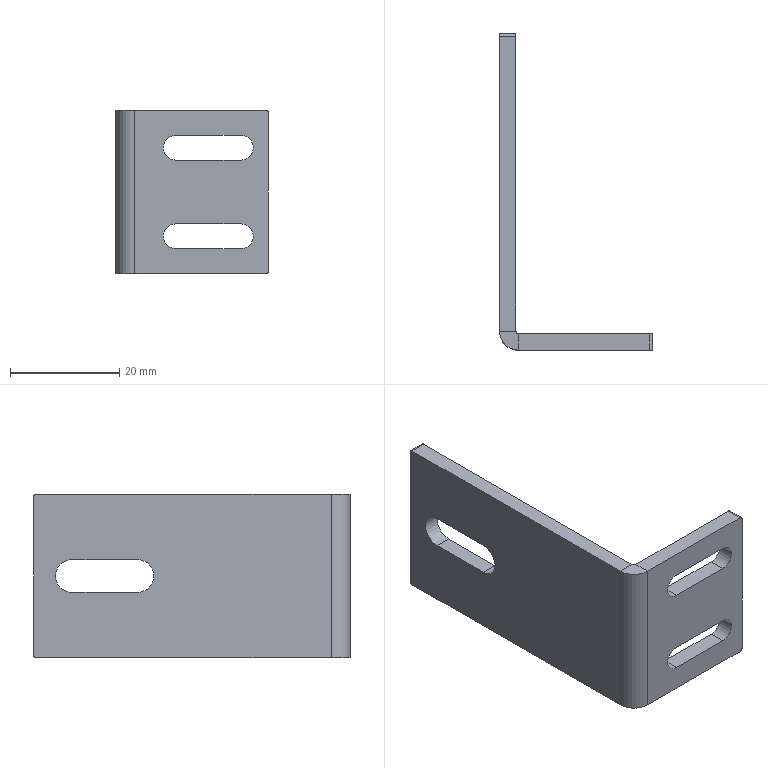Part | SolidWorks | features ICE 2, Fillet 1, FlatPattern 1, SMBaseFlange 1, SheetMetal 1 | 1 solid | 30 faces | box 28 x 58 x 30 mm | volume 6672 mm3 | plane 18 | cylinder 12 | commonest cylinder face diameters 1 x5 4.5 x4 6 x2 7 x1
STEP:
#1=CARTESIAN_POINT('',(0.5,0.,30.));
#2=VERTEX_POINT('',#1);
#3=CARTESIAN_POINT('',(0.5,-3.,30.));
#4=VERTEX_POINT('',#3);
#5=CARTESIAN_POINT('',(0.5,0.,30.));
#6=DIRECTION('',(0.,-1.,0.));
#7=VECTOR('',#6,1000.);
#8=LINE('',#5,#7);
#9=EDGE_CURVE('',#2,#4,#8,.T.);
#10=ORIENTED_EDGE('',*,*,#9,.F.);
#11=CARTESIAN_POINT('',(0.,0.5,30.));
#12=VERTEX_POINT('',#11);
#13=CARTESIAN_POINT('',(0.5,0.5,30.));
#14=DIRECTION('',(0.,0.,1.));
#15=DIRECTION('',(-1.,0.,0.));
#16=AXIS2_PLACEMENT_3D('',#13,#14,#15);
#17=CIRCLE('',#16,0.5);
#18=EDGE_CURVE('',#12,#2,#17,.T.);
#19=ORIENTED_EDGE('',*,*,#18,.F.);
#20=CARTESIAN_POINT('',(-3.,0.5,30.));
#21=VERTEX_POINT('',#20);
#22=CARTESIAN_POINT('',(-3.,0.5,30.));
#23=DIRECTION('',(1.,0.,0.));
#24=VECTOR('',#23,1000.);
#25=LINE('',#22,#24);
#26=EDGE_CURVE('',#21,#12,#25,.T.);
#27=ORIENTED_EDGE('',*,*,#26,.F.);
#28=CARTESIAN_POINT('',(0.5,0.5,30.));
#29=DIRECTION('',(0.,0.,1.));
#30=DIRECTION('',(1.,0.,0.));
#31=AXIS2_PLACEMENT_3D('',#28,#29,#30);
#32=CIRCLE('',#31,3.5);
#33=EDGE_CURVE('',#21,#4,#32,.T.);
#34=ORIENTED_EDGE('',*,*,#33,.T.);
#35=EDGE_LOOP('',(#10,#19,#27,#34));
#36=FACE_OUTER_BOUND('',#35,.T.);
#37=CARTESIAN_POINT('',(0.5,0.,30.));
#38=DIRECTION('',(0.,0.,1.));
#39=DIRECTION('',(1.,0.,0.));
#40=AXIS2_PLACEMENT_3D('',#37,#38,#39);
#41=PLANE('',#40);
#42=ADVANCED_FACE('',(#36),#41,.T.);
#43=CARTESIAN_POINT('',(24.5,-3.,30.));
#44=VERTEX_POINT('',#43);
#45=CARTESIAN_POINT('',(0.,-3.,30.));
#46=DIRECTION('',(1.,0.,0.));
#47=VECTOR('',#46,1000.);
#48=LINE('',#45,#47);
#49=EDGE_CURVE('',#4,#44,#48,.T.);
#50=ORIENTED_EDGE('',*,*,#49,.T.);
#51=CARTESIAN_POINT('',(24.5,0.,30.));
#52=VERTEX_POINT('',#51);
#53=CARTESIAN_POINT('',(24.5,0.5,30.));
#54=DIRECTION('',(0.,1.,0.));
#55=VECTOR('',#54,1000.);
#56=LINE('',#53,#55);
#57=EDGE_CURVE('',#44,#52,#56,.T.);
#58=ORIENTED_EDGE('',*,*,#57,.T.);
#59=CARTESIAN_POINT('',(0.,0.,30.));
#60=DIRECTION('',(1.,0.,0.));
#61=VECTOR('',#60,1000.);
#62=LINE('',#59,#61);
#63=EDGE_CURVE('',#2,#52,#62,.T.);
#64=ORIENTED_EDGE('',*,*,#63,.F.);
#65=ORIENTED_EDGE('',*,*,#9,.T.);
#66=EDGE_LOOP('',(#50,#58,#64,#65));
#67=FACE_OUTER_BOUND('',#66,.T.);
#68=CARTESIAN_POINT('',(-3.,0.5,30.));
#69=DIRECTION('',(0.,0.,1.));
#70=DIRECTION('',(1.,0.,0.));
#71=AXIS2_PLACEMENT_3D('',#68,#69,#70);
#72=PLANE('',#71);
#73=ADVANCED_FACE('',(#67),#72,.T.);
#74=CARTESIAN_POINT('',(0.,0.5,0.));
#75=VERTEX_POINT('',#74);
#76=CARTESIAN_POINT('',(-3.,0.5,0.));
#77=VERTEX_POINT('',#76);
#78=CARTESIAN_POINT('',(0.,0.5,0.));
#79=DIRECTION('',(-1.,0.,0.));
#80=VECTOR('',#79,1000.);
#81=LINE('',#78,#80);
#82=EDGE_CURVE('',#75,#77,#81,.T.);
#83=ORIENTED_EDGE('',*,*,#82,.F.);
#84=CARTESIAN_POINT('',(0.5,0.,0.));
#85=VERTEX_POINT('',#84);
#86=CARTESIAN_POINT('',(0.5,0.5,0.));
#87=DIRECTION('',(0.,0.,1.));
#88=DIRECTION('',(-1.,0.,0.));
#89=AXIS2_PLACEMENT_3D('',#86,#87,#88);
#90=CIRCLE('',#89,0.5);
#91=EDGE_CURVE('',#75,#85,#90,.T.);
#92=ORIENTED_EDGE('',*,*,#91,.T.);
#93=CARTESIAN_POINT('',(0.5,-3.,0.));
#94=VERTEX_POINT('',#93);
#95=CARTESIAN_POINT('',(0.5,-3.,0.));
#96=DIRECTION('',(0.,1.,0.));
#97=VECTOR('',#96,1000.);
#98=LINE('',#95,#97);
#99=EDGE_CURVE('',#94,#85,#98,.T.);
#100=ORIENTED_EDGE('',*,*,#99,.F.);
#101=CARTESIAN_POINT('',(0.5,0.5,0.));
#102=DIRECTION('',(0.,0.,1.));
#103=DIRECTION('',(1.,0.,0.));
#104=AXIS2_PLACEMENT_3D('',#101,#102,#103);
#105=CIRCLE('',#104,3.5);
#106=EDGE_CURVE('',#77,#94,#105,.T.);
#107=ORIENTED_EDGE('',*,*,#106,.F.);
#108=EDGE_LOOP('',(#83,#92,#100,#107));
#109=FACE_OUTER_BOUND('',#108,.T.);
#110=CARTESIAN_POINT('',(0.,0.5,0.));
#111=DIRECTION('',(0.,0.,-1.));
#112=DIRECTION('',(-1.,0.,0.));
#113=AXIS2_PLACEMENT_3D('',#110,#111,#112);
#114=PLANE('',#113);
#115=ADVANCED_FACE('',(#109),#114,.T.);
#116=CARTESIAN_POINT('',(-3.,54.5,0.));
#117=VERTEX_POINT('',#116);
#118=CARTESIAN_POINT('',(-3.,0.,0.));
#119=DIRECTION('',(0.,-1.,0.));
#120=VECTOR('',#119,1000.);
#121=LINE('',#118,#120);
#122=EDGE_CURVE('',#117,#77,#121,.T.);
#123=ORIENTED_EDGE('',*,*,#122,.F.);
#124=CARTESIAN_POINT('',(0.,54.5,0.));
#125=VERTEX_POINT('',#124);
#126=CARTESIAN_POINT('',(0.5,54.5,0.));
#127=DIRECTION('',(1.,0.,0.));
#128=VECTOR('',#127,1000.);
#129=LINE('',#126,#128);
#130=EDGE_CURVE('',#117,#125,#129,.T.);
#131=ORIENTED_EDGE('',*,*,#130,.T.);
#132=CARTESIAN_POINT('',(0.,0.,0.));
#133=DIRECTION('',(0.,-1.,0.));
#134=VECTOR('',#133,1000.);
#135=LINE('',#132,#134);
#136=EDGE_CURVE('',#125,#75,#135,.T.);
#137=ORIENTED_EDGE('',*,*,#136,.T.);
#138=ORIENTED_EDGE('',*,*,#82,.T.);
#139=EDGE_LOOP('',(#123,#131,#137,#138));
#140=FACE_OUTER_BOUND('',#139,.T.);
#141=CARTESIAN_POINT('',(0.5,-3.,0.));
#142=DIRECTION('',(0.,0.,-1.));
#143=DIRECTION('',(-1.,0.,0.));
#144=AXIS2_PLACEMENT_3D('',#141,#142,#143);
#145=PLANE('',#144);
#146=ADVANCED_FACE('',(#140),#145,.T.);
#147=CARTESIAN_POINT('',(8.,-3.,4.646));
#148=VERTEX_POINT('',#147);
#149=CARTESIAN_POINT('',(20.,-3.,4.646));
#150=VERTEX_POINT('',#149);
#151=CARTESIAN_POINT('',(8.,-3.,4.646));
#152=DIRECTION('',(1.,0.,0.));
#153=VECTOR('',#152,1000.);
#154=LINE('',#151,#153);
#155=EDGE_CURVE('',#148,#150,#154,.T.);
#156=ORIENTED_EDGE('',*,*,#155,.F.);
#157=CARTESIAN_POINT('',(8.,-3.,9.146));
#158=VERTEX_POINT('',#157);
#159=CARTESIAN_POINT('',(8.,-3.,6.896));
#160=DIRECTION('',(0.,-1.,0.));
#161=DIRECTION('',(0.,0.,1.));
#162=AXIS2_PLACEMENT_3D('',#159,#160,#161);
#163=CIRCLE('',#162,2.25);
#164=EDGE_CURVE('',#158,#148,#163,.T.);
#165=ORIENTED_EDGE('',*,*,#164,.F.);
#166=CARTESIAN_POINT('',(20.,-3.,9.146));
#167=VERTEX_POINT('',#166);
#168=CARTESIAN_POINT('',(8.,-3.,9.146));
#169=DIRECTION('',(-1.,0.,0.));
#170=VECTOR('',#169,1000.);
#171=LINE('',#168,#170);
#172=EDGE_CURVE('',#167,#158,#171,.T.);
#173=ORIENTED_EDGE('',*,*,#172,.F.);
#174=CARTESIAN_POINT('',(20.,-3.,6.896));
#175=DIRECTION('',(0.,-1.,0.));
#176=DIRECTION('',(0.,0.,1.));
#177=AXIS2_PLACEMENT_3D('',#174,#175,#176);
#178=CIRCLE('',#177,2.25);
#179=EDGE_CURVE('',#150,#167,#178,.T.);
#180=ORIENTED_EDGE('',*,*,#179,.F.);
#181=EDGE_LOOP('',(#156,#165,#173,#180));
#182=FACE_BOUND('',#181,.T.);
#183=CARTESIAN_POINT('',(8.,-3.,20.854));
#184=VERTEX_POINT('',#183);
#185=CARTESIAN_POINT('',(20.,-3.,20.854));
#186=VERTEX_POINT('',#185);
#187=CARTESIAN_POINT('',(8.,-3.,20.854));
#188=DIRECTION('',(1.,0.,0.));
#189=VECTOR('',#188,1000.);
#190=LINE('',#187,#189);
#191=EDGE_CURVE('',#184,#186,#190,.T.);
#192=ORIENTED_EDGE('',*,*,#191,.F.);
#193=CARTESIAN_POINT('',(8.,-3.,25.354));
#194=VERTEX_POINT('',#193);
#195=CARTESIAN_POINT('',(8.,-3.,23.104));
#196=DIRECTION('',(0.,-1.,0.));
#197=DIRECTION('',(0.,0.,-1.));
#198=AXIS2_PLACEMENT_3D('',#195,#196,#197);
#199=CIRCLE('',#198,2.25);
#200=EDGE_CURVE('',#194,#184,#199,.T.);
#201=ORIENTED_EDGE('',*,*,#200,.F.);
#202=CARTESIAN_POINT('',(20.,-3.,25.354));
#203=VERTEX_POINT('',#202);
#204=CARTESIAN_POINT('',(8.,-3.,25.354));
#205=DIRECTION('',(-1.,0.,0.));
#206=VECTOR('',#205,1000.);
#207=LINE('',#204,#206);
#208=EDGE_CURVE('',#203,#194,#207,.T.);
#209=ORIENTED_EDGE('',*,*,#208,.F.);
#210=CARTESIAN_POINT('',(20.,-3.,23.104));
#211=DIRECTION('',(0.,-1.,0.));
#212=DIRECTION('',(0.,0.,-1.));
#213=AXIS2_PLACEMENT_3D('',#210,#211,#212);
#214=CIRCLE('',#213,2.25);
#215=EDGE_CURVE('',#186,#203,#214,.T.);
#216=ORIENTED_EDGE('',*,*,#215,.F.);
#217=EDGE_LOOP('',(#192,#201,#209,#216));
#218=FACE_BOUND('',#217,.T.);
#219=CARTESIAN_POINT('',(24.5,-3.,0.));
#220=VERTEX_POINT('',#219);
#221=CARTESIAN_POINT('',(0.,-3.,0.));
#222=DIRECTION('',(1.,0.,0.));
#223=VECTOR('',#222,1000.);
#224=LINE('',#221,#223);
#225=EDGE_CURVE('',#94,#220,#224,.T.);
#226=ORIENTED_EDGE('',*,*,#225,.T.);
#227=CARTESIAN_POINT('',(25.,-3.,0.5));
#228=VERTEX_POINT('',#227);
#229=CARTESIAN_POINT('',(24.5,-3.,0.5));
#230=DIRECTION('',(0.,-1.,0.));
#231=DIRECTION('',(0.,0.,1.));
#232=AXIS2_PLACEMENT_3D('',#229,#230,#231);
#233=CIRCLE('',#232,0.5);
#234=EDGE_CURVE('',#220,#228,#233,.T.);
#235=ORIENTED_EDGE('',*,*,#234,.T.);
#236=CARTESIAN_POINT('',(25.,-3.,29.5));
#237=VERTEX_POINT('',#236);
#238=CARTESIAN_POINT('',(25.,-3.,30.));
#239=DIRECTION('',(0.,0.,-1.));
#240=VECTOR('',#239,1000.);
#241=LINE('',#238,#240);
#242=EDGE_CURVE('',#237,#228,#241,.T.);
#243=ORIENTED_EDGE('',*,*,#242,.F.);
#244=CARTESIAN_POINT('',(24.5,-3.,29.5));
#245=DIRECTION('',(0.,-1.,0.));
#246=DIRECTION('',(0.,0.,1.));
#247=AXIS2_PLACEMENT_3D('',#244,#245,#246);
#248=CIRCLE('',#247,0.5);
#249=EDGE_CURVE('',#237,#44,#248,.T.);
#250=ORIENTED_EDGE('',*,*,#249,.T.);
#251=ORIENTED_EDGE('',*,*,#49,.F.);
#252=CARTESIAN_POINT('',(0.5,-3.,30.));
#253=DIRECTION('',(0.,0.,-1.));
#254=VECTOR('',#253,1000.);
#255=LINE('',#252,#254);
#256=EDGE_CURVE('',#4,#94,#255,.T.);
#257=ORIENTED_EDGE('',*,*,#256,.T.);
#258=EDGE_LOOP('',(#226,#235,#243,#250,#251,#257));
#259=FACE_OUTER_BOUND('',#258,.T.);
#260=CARTESIAN_POINT('',(0.,-3.,30.));
#261=DIRECTION('',(0.,1.,0.));
#262=DIRECTION('',(0.,0.,1.));
#263=AXIS2_PLACEMENT_3D('',#260,#261,#262);
#264=PLANE('',#263);
#265=ADVANCED_FACE('',(#182,#218,#259),#264,.F.);
#266=ORIENTED_EDGE('',*,*,#242,.T.);
#267=CARTESIAN_POINT('',(25.,0.,0.5));
#268=VERTEX_POINT('',#267);
#269=CARTESIAN_POINT('',(25.,0.,0.5));
#270=DIRECTION('',(0.,1.,0.));
#271=VECTOR('',#270,1000.);
#272=LINE('',#269,#271);
#273=EDGE_CURVE('',#228,#268,#272,.T.);
#274=ORIENTED_EDGE('',*,*,#273,.T.);
#275=CARTESIAN_POINT('',(25.,0.,29.5));
#276=VERTEX_POINT('',#275);
#277=CARTESIAN_POINT('',(25.,0.,30.));
#278=DIRECTION('',(0.,0.,-1.));
#279=VECTOR('',#278,1000.);
#280=LINE('',#277,#279);
#281=EDGE_CURVE('',#276,#268,#280,.T.);
#282=ORIENTED_EDGE('',*,*,#281,.F.);
#283=CARTESIAN_POINT('',(25.,0.,29.5));
#284=DIRECTION('',(0.,-1.,0.));
#285=VECTOR('',#284,1000.);
#286=LINE('',#283,#285);
#287=EDGE_CURVE('',#276,#237,#286,.T.);
#288=ORIENTED_EDGE('',*,*,#287,.T.);
#289=EDGE_LOOP('',(#266,#274,#282,#288));
#290=FACE_OUTER_BOUND('',#289,.T.);
#291=CARTESIAN_POINT('',(25.,0.,30.));
#292=DIRECTION('',(1.,0.,0.));
#293=DIRECTION('',(0.,0.,-1.));
#294=AXIS2_PLACEMENT_3D('',#291,#292,#293);
#295=PLANE('',#294);
#296=ADVANCED_FACE('',(#290),#295,.T.);
#297=CARTESIAN_POINT('',(8.,0.,4.646));
#298=VERTEX_POINT('',#297);
#299=CARTESIAN_POINT('',(8.,0.,9.146));
#300=VERTEX_POINT('',#299);
#301=CARTESIAN_POINT('',(8.,0.,6.896));
#302=DIRECTION('',(0.,1.,0.));
#303=DIRECTION('',(0.,0.,1.));
#304=AXIS2_PLACEMENT_3D('',#301,#302,#303);
#305=CIRCLE('',#304,2.25);
#306=EDGE_CURVE('',#298,#300,#305,.T.);
#307=ORIENTED_EDGE('',*,*,#306,.F.);
#308=CARTESIAN_POINT('',(20.,0.,4.646));
#309=VERTEX_POINT('',#308);
#310=CARTESIAN_POINT('',(0.,0.,4.646));
#311=DIRECTION('',(-1.,0.,0.));
#312=VECTOR('',#311,1000.);
#313=LINE('',#310,#312);
#314=EDGE_CURVE('',#309,#298,#313,.T.);
#315=ORIENTED_EDGE('',*,*,#314,.F.);
#316=CARTESIAN_POINT('',(20.,0.,9.146));
#317=VERTEX_POINT('',#316);
#318=CARTESIAN_POINT('',(20.,0.,6.896));
#319=DIRECTION('',(0.,1.,0.));
#320=DIRECTION('',(0.,0.,1.));
#321=AXIS2_PLACEMENT_3D('',#318,#319,#320);
#322=CIRCLE('',#321,2.25);
#323=EDGE_CURVE('',#317,#309,#322,.T.);
#324=ORIENTED_EDGE('',*,*,#323,.F.);
#325=CARTESIAN_POINT('',(0.,0.,9.146));
#326=DIRECTION('',(1.,0.,0.));
#327=VECTOR('',#326,1000.);
#328=LINE('',#325,#327);
#329=EDGE_CURVE('',#300,#317,#328,.T.);
#330=ORIENTED_EDGE('',*,*,#329,.F.);
#331=EDGE_LOOP('',(#307,#315,#324,#330));
#332=FACE_BOUND('',#331,.T.);
#333=CARTESIAN_POINT('',(8.,0.,20.854));
#334=VERTEX_POINT('',#333);
#335=CARTESIAN_POINT('',(8.,0.,25.354));
#336=VERTEX_POINT('',#335);
#337=CARTESIAN_POINT('',(8.,0.,23.104));
#338=DIRECTION('',(0.,1.,0.));
#339=DIRECTION('',(0.,0.,1.));
#340=AXIS2_PLACEMENT_3D('',#337,#338,#339);
#341=CIRCLE('',#340,2.25);
#342=EDGE_CURVE('',#334,#336,#341,.T.);
#343=ORIENTED_EDGE('',*,*,#342,.F.);
#344=CARTESIAN_POINT('',(20.,0.,20.854));
#345=VERTEX_POINT('',#344);
#346=CARTESIAN_POINT('',(0.,0.,20.854));
#347=DIRECTION('',(-1.,0.,0.));
#348=VECTOR('',#347,1000.);
#349=LINE('',#346,#348);
#350=EDGE_CURVE('',#345,#334,#349,.T.);
#351=ORIENTED_EDGE('',*,*,#350,.F.);
#352=CARTESIAN_POINT('',(20.,0.,25.354));
#353=VERTEX_POINT('',#352);
#354=CARTESIAN_POINT('',(20.,0.,23.104));
#355=DIRECTION('',(0.,1.,0.));
#356=DIRECTION('',(0.,0.,1.));
#357=AXIS2_PLACEMENT_3D('',#354,#355,#356);
#358=CIRCLE('',#357,2.25);
#359=EDGE_CURVE('',#353,#345,#358,.T.);
#360=ORIENTED_EDGE('',*,*,#359,.F.);
#361=CARTESIAN_POINT('',(0.,0.,25.354));
#362=DIRECTION('',(1.,0.,0.));
#363=VECTOR('',#362,1000.);
#364=LINE('',#361,#363);
#365=EDGE_CURVE('',#336,#353,#364,.T.);
#366=ORIENTED_EDGE('',*,*,#365,.F.);
#367=EDGE_LOOP('',(#343,#351,#360,#366));
#368=FACE_BOUND('',#367,.T.);
#369=ORIENTED_EDGE('',*,*,#281,.T.);
#370=CARTESIAN_POINT('',(24.5,0.,0.));
#371=VERTEX_POINT('',#370);
#372=CARTESIAN_POINT('',(24.5,0.,0.5));
#373=DIRECTION('',(0.,1.,0.));
#374=DIRECTION('',(0.,0.,1.));
#375=AXIS2_PLACEMENT_3D('',#372,#373,#374);
#376=CIRCLE('',#375,0.5);
#377=EDGE_CURVE('',#268,#371,#376,.T.);
#378=ORIENTED_EDGE('',*,*,#377,.T.);
#379=CARTESIAN_POINT('',(0.,0.,0.));
#380=DIRECTION('',(1.,0.,0.));
#381=VECTOR('',#380,1000.);
#382=LINE('',#379,#381);
#383=EDGE_CURVE('',#85,#371,#382,.T.);
#384=ORIENTED_EDGE('',*,*,#383,.F.);
#385=CARTESIAN_POINT('',(0.5,0.,30.));
#386=DIRECTION('',(0.,0.,-1.));
#387=VECTOR('',#386,1000.);
#388=LINE('',#385,#387);
#389=EDGE_CURVE('',#2,#85,#388,.T.);
#390=ORIENTED_EDGE('',*,*,#389,.F.);
#391=ORIENTED_EDGE('',*,*,#63,.T.);
#392=CARTESIAN_POINT('',(24.5,0.,29.5));
#393=DIRECTION('',(0.,1.,0.));
#394=DIRECTION('',(0.,0.,1.));
#395=AXIS2_PLACEMENT_3D('',#392,#393,#394);
#396=CIRCLE('',#395,0.5);
#397=EDGE_CURVE('',#52,#276,#396,.T.);
#398=ORIENTED_EDGE('',*,*,#397,.T.);
#399=EDGE_LOOP('',(#369,#378,#384,#390,#391,#398));
#400=FACE_OUTER_BOUND('',#399,.T.);
#401=CARTESIAN_POINT('',(0.,0.,30.));
#402=DIRECTION('',(0.,1.,0.));
#403=DIRECTION('',(0.,0.,1.));
#404=AXIS2_PLACEMENT_3D('',#401,#402,#403);
#405=PLANE('',#404);
#406=ADVANCED_FACE('',(#332,#368,#400),#405,.T.);
#407=ORIENTED_EDGE('',*,*,#91,.F.);
#408=CARTESIAN_POINT('',(0.,0.5,30.));
#409=DIRECTION('',(0.,0.,-1.));
#410=VECTOR('',#409,1000.);
#411=LINE('',#408,#410);
#412=EDGE_CURVE('',#12,#75,#411,.T.);
#413=ORIENTED_EDGE('',*,*,#412,.F.);
#414=ORIENTED_EDGE('',*,*,#18,.T.);
#415=ORIENTED_EDGE('',*,*,#389,.T.);
#416=EDGE_LOOP('',(#407,#413,#414,#415));
#417=FACE_OUTER_BOUND('',#416,.T.);
#418=CARTESIAN_POINT('',(0.5,0.5,30.));
#419=DIRECTION('',(0.,0.,-1.));
#420=DIRECTION('',(-1.,0.,0.));
#421=AXIS2_PLACEMENT_3D('',#418,#419,#420);
#422=CYLINDRICAL_SURFACE('',#421,0.5);
#423=ADVANCED_FACE('',(#417),#422,.F.);
#424=CARTESIAN_POINT('',(0.,48.,12.));
#425=VERTEX_POINT('',#424);
#426=CARTESIAN_POINT('',(0.,48.,18.));
#427=VERTEX_POINT('',#426);
#428=CARTESIAN_POINT('',(0.,48.,15.));
#429=DIRECTION('',(1.,0.,0.));
#430=DIRECTION('',(0.,0.,-1.));
#431=AXIS2_PLACEMENT_3D('',#428,#429,#430);
#432=CIRCLE('',#431,3.);
#433=EDGE_CURVE('',#425,#427,#432,.T.);
#434=ORIENTED_EDGE('',*,*,#433,.F.);
#435=CARTESIAN_POINT('',(0.,36.,12.));
#436=VERTEX_POINT('',#435);
#437=CARTESIAN_POINT('',(0.,0.,12.));
#438=DIRECTION('',(0.,1.,0.));
#439=VECTOR('',#438,1000.);
#440=LINE('',#437,#439);
#441=EDGE_CURVE('',#436,#425,#440,.T.);
#442=ORIENTED_EDGE('',*,*,#441,.F.);
#443=CARTESIAN_POINT('',(0.,36.,18.));
#444=VERTEX_POINT('',#443);
#445=CARTESIAN_POINT('',(0.,36.,15.));
#446=DIRECTION('',(1.,0.,0.));
#447=DIRECTION('',(0.,0.,-1.));
#448=AXIS2_PLACEMENT_3D('',#445,#446,#447);
#449=CIRCLE('',#448,3.);
#450=EDGE_CURVE('',#444,#436,#449,.T.);
#451=ORIENTED_EDGE('',*,*,#450,.F.);
#452=CARTESIAN_POINT('',(0.,0.,18.));
#453=DIRECTION('',(0.,-1.,0.));
#454=VECTOR('',#453,1000.);
#455=LINE('',#452,#454);
#456=EDGE_CURVE('',#427,#444,#455,.T.);
#457=ORIENTED_EDGE('',*,*,#456,.F.);
#458=EDGE_LOOP('',(#434,#442,#451,#457));
#459=FACE_BOUND('',#458,.T.);
#460=CARTESIAN_POINT('',(0.,55.,29.5));
#461=VERTEX_POINT('',#460);
#462=CARTESIAN_POINT('',(0.,55.,0.5));
#463=VERTEX_POINT('',#462);
#464=CARTESIAN_POINT('',(0.,55.,30.));
#465=DIRECTION('',(0.,0.,-1.));
#466=VECTOR('',#465,1000.);
#467=LINE('',#464,#466);
#468=EDGE_CURVE('',#461,#463,#467,.T.);
#469=ORIENTED_EDGE('',*,*,#468,.F.);
#470=CARTESIAN_POINT('',(0.,54.5,30.));
#471=VERTEX_POINT('',#470);
#472=CARTESIAN_POINT('',(0.,54.5,29.5));
#473=DIRECTION('',(1.,0.,0.));
#474=DIRECTION('',(0.,0.,-1.));
#475=AXIS2_PLACEMENT_3D('',#472,#473,#474);
#476=CIRCLE('',#475,0.5);
#477=EDGE_CURVE('',#461,#471,#476,.T.);
#478=ORIENTED_EDGE('',*,*,#477,.T.);
#479=CARTESIAN_POINT('',(0.,0.,30.));
#480=DIRECTION('',(0.,-1.,0.));
#481=VECTOR('',#480,1000.);
#482=LINE('',#479,#481);
#483=EDGE_CURVE('',#471,#12,#482,.T.);
#484=ORIENTED_EDGE('',*,*,#483,.T.);
#485=ORIENTED_EDGE('',*,*,#412,.T.);
#486=ORIENTED_EDGE('',*,*,#136,.F.);
#487=CARTESIAN_POINT('',(0.,54.5,0.5));
#488=DIRECTION('',(1.,0.,0.));
#489=DIRECTION('',(0.,0.,-1.));
#490=AXIS2_PLACEMENT_3D('',#487,#488,#489);
#491=CIRCLE('',#490,0.5);
#492=EDGE_CURVE('',#125,#463,#491,.T.);
#493=ORIENTED_EDGE('',*,*,#492,.T.);
#494=EDGE_LOOP('',(#469,#478,#484,#485,#486,#493));
#495=FACE_OUTER_BOUND('',#494,.T.);
#496=CARTESIAN_POINT('',(0.,0.,30.));
#497=DIRECTION('',(1.,0.,0.));
#498=DIRECTION('',(0.,0.,-1.));
#499=AXIS2_PLACEMENT_3D('',#496,#497,#498);
#500=PLANE('',#499);
#501=ADVANCED_FACE('',(#459,#495),#500,.T.);
#502=CARTESIAN_POINT('',(-3.,55.,29.5));
#503=VERTEX_POINT('',#502);
#504=CARTESIAN_POINT('',(-3.,55.,0.5));
#505=VERTEX_POINT('',#504);
#506=CARTESIAN_POINT('',(-3.,55.,30.));
#507=DIRECTION('',(0.,0.,-1.));
#508=VECTOR('',#507,1000.);
#509=LINE('',#506,#508);
#510=EDGE_CURVE('',#503,#505,#509,.T.);
#511=ORIENTED_EDGE('',*,*,#510,.F.);
#512=CARTESIAN_POINT('',(0.,55.,29.5));
#513=DIRECTION('',(1.,0.,0.));
#514=VECTOR('',#513,1000.);
#515=LINE('',#512,#514);
#516=EDGE_CURVE('',#503,#461,#515,.T.);
#517=ORIENTED_EDGE('',*,*,#516,.T.);
#518=ORIENTED_EDGE('',*,*,#468,.T.);
#519=CARTESIAN_POINT('',(-3.,55.,0.5));
#520=DIRECTION('',(-1.,0.,0.));
#521=VECTOR('',#520,1000.);
#522=LINE('',#519,#521);
#523=EDGE_CURVE('',#463,#505,#522,.T.);
#524=ORIENTED_EDGE('',*,*,#523,.T.);
#525=EDGE_LOOP('',(#511,#517,#518,#524));
#526=FACE_OUTER_BOUND('',#525,.T.);
#527=CARTESIAN_POINT('',(-3.,55.,30.));
#528=DIRECTION('',(0.,1.,0.));
#529=DIRECTION('',(0.,0.,1.));
#530=AXIS2_PLACEMENT_3D('',#527,#528,#529);
#531=PLANE('',#530);
#532=ADVANCED_FACE('',(#526),#531,.T.);
#533=CARTESIAN_POINT('',(-3.,48.,12.));
#534=VERTEX_POINT('',#533);
#535=CARTESIAN_POINT('',(-3.,36.,12.));
#536=VERTEX_POINT('',#535);
#537=CARTESIAN_POINT('',(-3.,48.,12.));
#538=DIRECTION('',(0.,-1.,0.));
#539=VECTOR('',#538,1000.);
#540=LINE('',#537,#539);
#541=EDGE_CURVE('',#534,#536,#540,.T.);
#542=ORIENTED_EDGE('',*,*,#541,.F.);
#543=CARTESIAN_POINT('',(-3.,48.,18.));
#544=VERTEX_POINT('',#543);
#545=CARTESIAN_POINT('',(-3.,48.,15.));
#546=DIRECTION('',(-1.,0.,0.));
#547=DIRECTION('',(0.,0.,1.));
#548=AXIS2_PLACEMENT_3D('',#545,#546,#547);
#549=CIRCLE('',#548,3.);
#550=EDGE_CURVE('',#544,#534,#549,.T.);
#551=ORIENTED_EDGE('',*,*,#550,.F.);
#552=CARTESIAN_POINT('',(-3.,36.,18.));
#553=VERTEX_POINT('',#552);
#554=CARTESIAN_POINT('',(-3.,48.,18.));
#555=DIRECTION('',(0.,1.,0.));
#556=VECTOR('',#555,1000.);
#557=LINE('',#554,#556);
#558=EDGE_CURVE('',#553,#544,#557,.T.);
#559=ORIENTED_EDGE('',*,*,#558,.F.);
#560=CARTESIAN_POINT('',(-3.,36.,15.));
#561=DIRECTION('',(-1.,0.,0.));
#562=DIRECTION('',(0.,0.,1.));
#563=AXIS2_PLACEMENT_3D('',#560,#561,#562);
#564=CIRCLE('',#563,3.);
#565=EDGE_CURVE('',#536,#553,#564,.T.);
#566=ORIENTED_EDGE('',*,*,#565,.F.);
#567=EDGE_LOOP('',(#542,#551,#559,#566));
#568=FACE_BOUND('',#567,.T.);
#569=CARTESIAN_POINT('',(-3.,54.5,30.));
#570=VERTEX_POINT('',#569);
#571=CARTESIAN_POINT('',(-3.,0.,30.));
#572=DIRECTION('',(0.,-1.,0.));
#573=VECTOR('',#572,1000.);
#574=LINE('',#571,#573);
#575=EDGE_CURVE('',#570,#21,#574,.T.);
#576=ORIENTED_EDGE('',*,*,#575,.F.);
#577=CARTESIAN_POINT('',(-3.,54.5,29.5));
#578=DIRECTION('',(-1.,0.,0.));
#579=DIRECTION('',(0.,0.,-1.));
#580=AXIS2_PLACEMENT_3D('',#577,#578,#579);
#581=CIRCLE('',#580,0.5);
#582=EDGE_CURVE('',#570,#503,#581,.T.);
#583=ORIENTED_EDGE('',*,*,#582,.T.);
#584=ORIENTED_EDGE('',*,*,#510,.T.);
#585=CARTESIAN_POINT('',(-3.,54.5,0.5));
#586=DIRECTION('',(-1.,0.,0.));
#587=DIRECTION('',(0.,0.,-1.));
#588=AXIS2_PLACEMENT_3D('',#585,#586,#587);
#589=CIRCLE('',#588,0.5);
#590=EDGE_CURVE('',#505,#117,#589,.T.);
#591=ORIENTED_EDGE('',*,*,#590,.T.);
#592=ORIENTED_EDGE('',*,*,#122,.T.);
#593=CARTESIAN_POINT('',(-3.,0.5,30.));
#594=DIRECTION('',(0.,0.,-1.));
#595=VECTOR('',#594,1000.);
#596=LINE('',#593,#595);
#597=EDGE_CURVE('',#21,#77,#596,.T.);
#598=ORIENTED_EDGE('',*,*,#597,.F.);
#599=EDGE_LOOP('',(#576,#583,#584,#591,#592,#598));
#600=FACE_OUTER_BOUND('',#599,.T.);
#601=CARTESIAN_POINT('',(-3.,0.,30.));
#602=DIRECTION('',(1.,0.,0.));
#603=DIRECTION('',(0.,0.,-1.));
#604=AXIS2_PLACEMENT_3D('',#601,#602,#603);
#605=PLANE('',#604);
#606=ADVANCED_FACE('',(#568,#600),#605,.F.);
#607=ORIENTED_EDGE('',*,*,#106,.T.);
#608=ORIENTED_EDGE('',*,*,#256,.F.);
#609=ORIENTED_EDGE('',*,*,#33,.F.);
#610=ORIENTED_EDGE('',*,*,#597,.T.);
#611=EDGE_LOOP('',(#607,#608,#609,#610));
#612=FACE_OUTER_BOUND('',#611,.T.);
#613=CARTESIAN_POINT('',(0.5,0.5,30.));
#614=DIRECTION('',(0.,0.,-1.));
#615=DIRECTION('',(-1.,0.,0.));
#616=AXIS2_PLACEMENT_3D('',#613,#614,#615);
#617=CYLINDRICAL_SURFACE('',#616,3.5);
#618=ADVANCED_FACE('',(#612),#617,.T.);
#619=ORIENTED_EDGE('',*,*,#483,.F.);
#620=CARTESIAN_POINT('',(-3.,54.5,30.));
#621=DIRECTION('',(-1.,0.,0.));
#622=VECTOR('',#621,1000.);
#623=LINE('',#620,#622);
#624=EDGE_CURVE('',#471,#570,#623,.T.);
#625=ORIENTED_EDGE('',*,*,#624,.T.);
#626=ORIENTED_EDGE('',*,*,#575,.T.);
#627=ORIENTED_EDGE('',*,*,#26,.T.);
#628=EDGE_LOOP('',(#619,#625,#626,#627));
#629=FACE_OUTER_BOUND('',#628,.T.);
#630=CARTESIAN_POINT('',(0.5,0.5,30.));
#631=DIRECTION('',(0.,0.,-1.));
#632=DIRECTION('',(-1.,0.,0.));
#633=AXIS2_PLACEMENT_3D('',#630,#631,#632);
#634=PLANE('',#633);
#635=ADVANCED_FACE('',(#629),#634,.F.);
#636=ORIENTED_EDGE('',*,*,#383,.T.);
#637=CARTESIAN_POINT('',(24.5,0.5,0.));
#638=DIRECTION('',(0.,-1.,0.));
#639=VECTOR('',#638,1000.);
#640=LINE('',#637,#639);
#641=EDGE_CURVE('',#371,#220,#640,.T.);
#642=ORIENTED_EDGE('',*,*,#641,.T.);
#643=ORIENTED_EDGE('',*,*,#225,.F.);
#644=ORIENTED_EDGE('',*,*,#99,.T.);
#645=EDGE_LOOP('',(#636,#642,#643,#644));
#646=FACE_OUTER_BOUND('',#645,.T.);
#647=CARTESIAN_POINT('',(0.5,0.5,0.));
#648=DIRECTION('',(0.,0.,-1.));
#649=DIRECTION('',(-1.,0.,0.));
#650=AXIS2_PLACEMENT_3D('',#647,#648,#649);
#651=PLANE('',#650);
#652=ADVANCED_FACE('',(#646),#651,.T.);
#653=ORIENTED_EDGE('',*,*,#342,.T.);
#654=CARTESIAN_POINT('',(8.,55.,25.354));
#655=DIRECTION('',(0.,-1.,0.));
#656=VECTOR('',#655,1000.);
#657=LINE('',#654,#656);
#658=EDGE_CURVE('',#336,#194,#657,.T.);
#659=ORIENTED_EDGE('',*,*,#658,.T.);
#660=ORIENTED_EDGE('',*,*,#200,.T.);
#661=CARTESIAN_POINT('',(8.,55.,20.854));
#662=DIRECTION('',(0.,-1.,0.));
#663=VECTOR('',#662,1000.);
#664=LINE('',#661,#663);
#665=EDGE_CURVE('',#334,#184,#664,.T.);
#666=ORIENTED_EDGE('',*,*,#665,.F.);
#667=EDGE_LOOP('',(#653,#659,#660,#666));
#668=FACE_OUTER_BOUND('',#667,.T.);
#669=CARTESIAN_POINT('',(8.,55.,23.104));
#670=DIRECTION('',(0.,-1.,0.));
#671=DIRECTION('',(0.,0.,-1.));
#672=AXIS2_PLACEMENT_3D('',#669,#670,#671);
#673=CYLINDRICAL_SURFACE('',#672,2.25);
#674=ADVANCED_FACE('',(#668),#673,.F.);
#675=ORIENTED_EDGE('',*,*,#365,.T.);
#676=CARTESIAN_POINT('',(20.,55.,25.354));
#677=DIRECTION('',(0.,-1.,0.));
#678=VECTOR('',#677,1000.);
#679=LINE('',#676,#678);
#680=EDGE_CURVE('',#353,#203,#679,.T.);
#681=ORIENTED_EDGE('',*,*,#680,.T.);
#682=ORIENTED_EDGE('',*,*,#208,.T.);
#683=ORIENTED_EDGE('',*,*,#658,.F.);
#684=EDGE_LOOP('',(#675,#681,#682,#683));
#685=FACE_OUTER_BOUND('',#684,.T.);
#686=CARTESIAN_POINT('',(8.,55.,25.354));
#687=DIRECTION('',(0.,0.,1.));
#688=DIRECTION('',(1.,0.,0.));
#689=AXIS2_PLACEMENT_3D('',#686,#687,#688);
#690=PLANE('',#689);
#691=ADVANCED_FACE('',(#685),#690,.F.);
#692=ORIENTED_EDGE('',*,*,#359,.T.);
#693=CARTESIAN_POINT('',(20.,55.,20.854));
#694=DIRECTION('',(0.,-1.,0.));
#695=VECTOR('',#694,1000.);
#696=LINE('',#693,#695);
#697=EDGE_CURVE('',#345,#186,#696,.T.);
#698=ORIENTED_EDGE('',*,*,#697,.T.);
#699=ORIENTED_EDGE('',*,*,#215,.T.);
#700=ORIENTED_EDGE('',*,*,#680,.F.);
#701=EDGE_LOOP('',(#692,#698,#699,#700));
#702=FACE_OUTER_BOUND('',#701,.T.);
#703=CARTESIAN_POINT('',(20.,55.,23.104));
#704=DIRECTION('',(0.,-1.,0.));
#705=DIRECTION('',(0.,0.,-1.));
#706=AXIS2_PLACEMENT_3D('',#703,#704,#705);
#707=CYLINDRICAL_SURFACE('',#706,2.25);
#708=ADVANCED_FACE('',(#702),#707,.F.);
#709=ORIENTED_EDGE('',*,*,#350,.T.);
#710=ORIENTED_EDGE('',*,*,#665,.T.);
#711=ORIENTED_EDGE('',*,*,#191,.T.);
#712=ORIENTED_EDGE('',*,*,#697,.F.);
#713=EDGE_LOOP('',(#709,#710,#711,#712));
#714=FACE_OUTER_BOUND('',#713,.T.);
#715=CARTESIAN_POINT('',(8.,55.,20.854));
#716=DIRECTION('',(0.,0.,-1.));
#717=DIRECTION('',(-1.,0.,0.));
#718=AXIS2_PLACEMENT_3D('',#715,#716,#717);
#719=PLANE('',#718);
#720=ADVANCED_FACE('',(#714),#719,.F.);
#721=ORIENTED_EDGE('',*,*,#306,.T.);
#722=CARTESIAN_POINT('',(8.,55.,9.146));
#723=DIRECTION('',(0.,-1.,0.));
#724=VECTOR('',#723,1000.);
#725=LINE('',#722,#724);
#726=EDGE_CURVE('',#300,#158,#725,.T.);
#727=ORIENTED_EDGE('',*,*,#726,.T.);
#728=ORIENTED_EDGE('',*,*,#164,.T.);
#729=CARTESIAN_POINT('',(8.,55.,4.646));
#730=DIRECTION('',(0.,-1.,0.));
#731=VECTOR('',#730,1000.);
#732=LINE('',#729,#731);
#733=EDGE_CURVE('',#298,#148,#732,.T.);
#734=ORIENTED_EDGE('',*,*,#733,.F.);
#735=EDGE_LOOP('',(#721,#727,#728,#734));
#736=FACE_OUTER_BOUND('',#735,.T.);
#737=CARTESIAN_POINT('',(8.,55.,6.896));
#738=DIRECTION('',(0.,-1.,0.));
#739=DIRECTION('',(0.,0.,-1.));
#740=AXIS2_PLACEMENT_3D('',#737,#738,#739);
#741=CYLINDRICAL_SURFACE('',#740,2.25);
#742=ADVANCED_FACE('',(#736),#741,.F.);
#743=ORIENTED_EDGE('',*,*,#329,.T.);
#744=CARTESIAN_POINT('',(20.,55.,9.146));
#745=DIRECTION('',(0.,-1.,0.));
#746=VECTOR('',#745,1000.);
#747=LINE('',#744,#746);
#748=EDGE_CURVE('',#317,#167,#747,.T.);
#749=ORIENTED_EDGE('',*,*,#748,.T.);
#750=ORIENTED_EDGE('',*,*,#172,.T.);
#751=ORIENTED_EDGE('',*,*,#726,.F.);
#752=EDGE_LOOP('',(#743,#749,#750,#751));
#753=FACE_OUTER_BOUND('',#752,.T.);
#754=CARTESIAN_POINT('',(8.,55.,9.146));
#755=DIRECTION('',(0.,0.,1.));
#756=DIRECTION('',(1.,0.,0.));
#757=AXIS2_PLACEMENT_3D('',#754,#755,#756);
#758=PLANE('',#757);
#759=ADVANCED_FACE('',(#753),#758,.F.);
#760=ORIENTED_EDGE('',*,*,#323,.T.);
#761=CARTESIAN_POINT('',(20.,55.,4.646));
#762=DIRECTION('',(0.,-1.,0.));
#763=VECTOR('',#762,1000.);
#764=LINE('',#761,#763);
#765=EDGE_CURVE('',#309,#150,#764,.T.);
#766=ORIENTED_EDGE('',*,*,#765,.T.);
#767=ORIENTED_EDGE('',*,*,#179,.T.);
#768=ORIENTED_EDGE('',*,*,#748,.F.);
#769=EDGE_LOOP('',(#760,#766,#767,#768));
#770=FACE_OUTER_BOUND('',#769,.T.);
#771=CARTESIAN_POINT('',(20.,55.,6.896));
#772=DIRECTION('',(0.,-1.,0.));
#773=DIRECTION('',(0.,0.,-1.));
#774=AXIS2_PLACEMENT_3D('',#771,#772,#773);
#775=CYLINDRICAL_SURFACE('',#774,2.25);
#776=ADVANCED_FACE('',(#770),#775,.F.);
#777=ORIENTED_EDGE('',*,*,#314,.T.);
#778=ORIENTED_EDGE('',*,*,#733,.T.);
#779=ORIENTED_EDGE('',*,*,#155,.T.);
#780=ORIENTED_EDGE('',*,*,#765,.F.);
#781=EDGE_LOOP('',(#777,#778,#779,#780));
#782=FACE_OUTER_BOUND('',#781,.T.);
#783=CARTESIAN_POINT('',(8.,55.,4.646));
#784=DIRECTION('',(0.,0.,-1.));
#785=DIRECTION('',(-1.,0.,0.));
#786=AXIS2_PLACEMENT_3D('',#783,#784,#785);
#787=PLANE('',#786);
#788=ADVANCED_FACE('',(#782),#787,.F.);
#789=ORIENTED_EDGE('',*,*,#433,.T.);
#790=CARTESIAN_POINT('',(25.,48.,18.));
#791=DIRECTION('',(-1.,0.,0.));
#792=VECTOR('',#791,1000.);
#793=LINE('',#790,#792);
#794=EDGE_CURVE('',#427,#544,#793,.T.);
#795=ORIENTED_EDGE('',*,*,#794,.T.);
#796=ORIENTED_EDGE('',*,*,#550,.T.);
#797=CARTESIAN_POINT('',(25.,48.,12.));
#798=DIRECTION('',(-1.,0.,0.));
#799=VECTOR('',#798,1000.);
#800=LINE('',#797,#799);
#801=EDGE_CURVE('',#425,#534,#800,.T.);
#802=ORIENTED_EDGE('',*,*,#801,.F.);
#803=EDGE_LOOP('',(#789,#795,#796,#802));
#804=FACE_OUTER_BOUND('',#803,.T.);
#805=CARTESIAN_POINT('',(25.,48.,15.));
#806=DIRECTION('',(-1.,0.,0.));
#807=DIRECTION('',(0.,0.,1.));
#808=AXIS2_PLACEMENT_3D('',#805,#806,#807);
#809=CYLINDRICAL_SURFACE('',#808,3.);
#810=ADVANCED_FACE('',(#804),#809,.F.);
#811=ORIENTED_EDGE('',*,*,#456,.T.);
#812=CARTESIAN_POINT('',(25.,36.,18.));
#813=DIRECTION('',(-1.,0.,0.));
#814=VECTOR('',#813,1000.);
#815=LINE('',#812,#814);
#816=EDGE_CURVE('',#444,#553,#815,.T.);
#817=ORIENTED_EDGE('',*,*,#816,.T.);
#818=ORIENTED_EDGE('',*,*,#558,.T.);
#819=ORIENTED_EDGE('',*,*,#794,.F.);
#820=EDGE_LOOP('',(#811,#817,#818,#819));
#821=FACE_OUTER_BOUND('',#820,.T.);
#822=CARTESIAN_POINT('',(25.,48.,18.));
#823=DIRECTION('',(0.,0.,1.));
#824=DIRECTION('',(0.,-1.,0.));
#825=AXIS2_PLACEMENT_3D('',#822,#823,#824);
#826=PLANE('',#825);
#827=ADVANCED_FACE('',(#821),#826,.F.);
#828=ORIENTED_EDGE('',*,*,#450,.T.);
#829=CARTESIAN_POINT('',(25.,36.,12.));
#830=DIRECTION('',(-1.,0.,0.));
#831=VECTOR('',#830,1000.);
#832=LINE('',#829,#831);
#833=EDGE_CURVE('',#436,#536,#832,.T.);
#834=ORIENTED_EDGE('',*,*,#833,.T.);
#835=ORIENTED_EDGE('',*,*,#565,.T.);
#836=ORIENTED_EDGE('',*,*,#816,.F.);
#837=EDGE_LOOP('',(#828,#834,#835,#836));
#838=FACE_OUTER_BOUND('',#837,.T.);
#839=CARTESIAN_POINT('',(25.,36.,15.));
#840=DIRECTION('',(-1.,0.,0.));
#841=DIRECTION('',(0.,0.,1.));
#842=AXIS2_PLACEMENT_3D('',#839,#840,#841);
#843=CYLINDRICAL_SURFACE('',#842,3.);
#844=ADVANCED_FACE('',(#838),#843,.F.);
#845=ORIENTED_EDGE('',*,*,#441,.T.);
#846=ORIENTED_EDGE('',*,*,#801,.T.);
#847=ORIENTED_EDGE('',*,*,#541,.T.);
#848=ORIENTED_EDGE('',*,*,#833,.F.);
#849=EDGE_LOOP('',(#845,#846,#847,#848));
#850=FACE_OUTER_BOUND('',#849,.T.);
#851=CARTESIAN_POINT('',(25.,48.,12.));
#852=DIRECTION('',(0.,0.,-1.));
#853=DIRECTION('',(0.,1.,0.));
#854=AXIS2_PLACEMENT_3D('',#851,#852,#853);
#855=PLANE('',#854);
#856=ADVANCED_FACE('',(#850),#855,.F.);
#857=ORIENTED_EDGE('',*,*,#377,.F.);
#858=ORIENTED_EDGE('',*,*,#273,.F.);
#859=ORIENTED_EDGE('',*,*,#234,.F.);
#860=ORIENTED_EDGE('',*,*,#641,.F.);
#861=EDGE_LOOP('',(#857,#858,#859,#860));
#862=FACE_OUTER_BOUND('',#861,.T.);
#863=CARTESIAN_POINT('',(24.5,0.5,0.5));
#864=DIRECTION('',(0.,-1.,0.));
#865=DIRECTION('',(0.,0.,-1.));
#866=AXIS2_PLACEMENT_3D('',#863,#864,#865);
#867=CYLINDRICAL_SURFACE('',#866,0.5);
#868=ADVANCED_FACE('',(#862),#867,.T.);
#869=ORIENTED_EDGE('',*,*,#397,.F.);
#870=ORIENTED_EDGE('',*,*,#57,.F.);
#871=ORIENTED_EDGE('',*,*,#249,.F.);
#872=ORIENTED_EDGE('',*,*,#287,.F.);
#873=EDGE_LOOP('',(#869,#870,#871,#872));
#874=FACE_OUTER_BOUND('',#873,.T.);
#875=CARTESIAN_POINT('',(24.5,0.,29.5));
#876=DIRECTION('',(0.,-1.,0.));
#877=DIRECTION('',(0.,0.,-1.));
#878=AXIS2_PLACEMENT_3D('',#875,#876,#877);
#879=CYLINDRICAL_SURFACE('',#878,0.5);
#880=ADVANCED_FACE('',(#874),#879,.T.);
#881=ORIENTED_EDGE('',*,*,#582,.F.);
#882=ORIENTED_EDGE('',*,*,#624,.F.);
#883=ORIENTED_EDGE('',*,*,#477,.F.);
#884=ORIENTED_EDGE('',*,*,#516,.F.);
#885=EDGE_LOOP('',(#881,#882,#883,#884));
#886=FACE_OUTER_BOUND('',#885,.T.);
#887=CARTESIAN_POINT('',(-3.,54.5,29.5));
#888=DIRECTION('',(-1.,0.,0.));
#889=DIRECTION('',(0.,0.,1.));
#890=AXIS2_PLACEMENT_3D('',#887,#888,#889);
#891=CYLINDRICAL_SURFACE('',#890,0.5);
#892=ADVANCED_FACE('',(#886),#891,.T.);
#893=ORIENTED_EDGE('',*,*,#590,.F.);
#894=ORIENTED_EDGE('',*,*,#523,.F.);
#895=ORIENTED_EDGE('',*,*,#492,.F.);
#896=ORIENTED_EDGE('',*,*,#130,.F.);
#897=EDGE_LOOP('',(#893,#894,#895,#896));
#898=FACE_OUTER_BOUND('',#897,.T.);
#899=CARTESIAN_POINT('',(0.5,54.5,0.5));
#900=DIRECTION('',(1.,0.,0.));
#901=DIRECTION('',(0.,0.,-1.));
#902=AXIS2_PLACEMENT_3D('',#899,#900,#901);
#903=CYLINDRICAL_SURFACE('',#902,0.5);
#904=ADVANCED_FACE('',(#898),#903,.T.);
#905=CLOSED_SHELL('',(#42,#73,#115,#146,#265,#296,#406,#423,#501,#532,#606,#618,#635,#652,#674,#691,#708,#720,#742,#759,#776,#788,#810,#827,#844,#856,#868,#880,#892,#904));
#906=MANIFOLD_SOLID_BREP('',#905);
#907=CARTESIAN_POINT('',(0.,0.,0.));
#908=DIRECTION('',(0.,0.,1.));
#909=DIRECTION('',(1.,0.,0.));
#910=AXIS2_PLACEMENT_3D('',#907,#908,#909);
#911=(LENGTH_UNIT()NAMED_UNIT(*)SI_UNIT(.MILLI.,.METRE.));
#912=UNCERTAINTY_MEASURE_WITH_UNIT(LENGTH_MEASURE(0.00001),#911,'','');
#913=(NAMED_UNIT(*)PLANE_ANGLE_UNIT()SI_UNIT($,.RADIAN.));
#914=(NAMED_UNIT(*)SI_UNIT($,.STERADIAN.)SOLID_ANGLE_UNIT());
#915=(GEOMETRIC_REPRESENTATION_CONTEXT(3)GLOBAL_UNCERTAINTY_ASSIGNED_CONTEXT((#912))GLOBAL_UNIT_ASSIGNED_CONTEXT((#911,#913,#914))REPRESENTATION_CONTEXT('',''));
#916=ADVANCED_BREP_SHAPE_REPRESENTATION('',(#906,#910),#915);